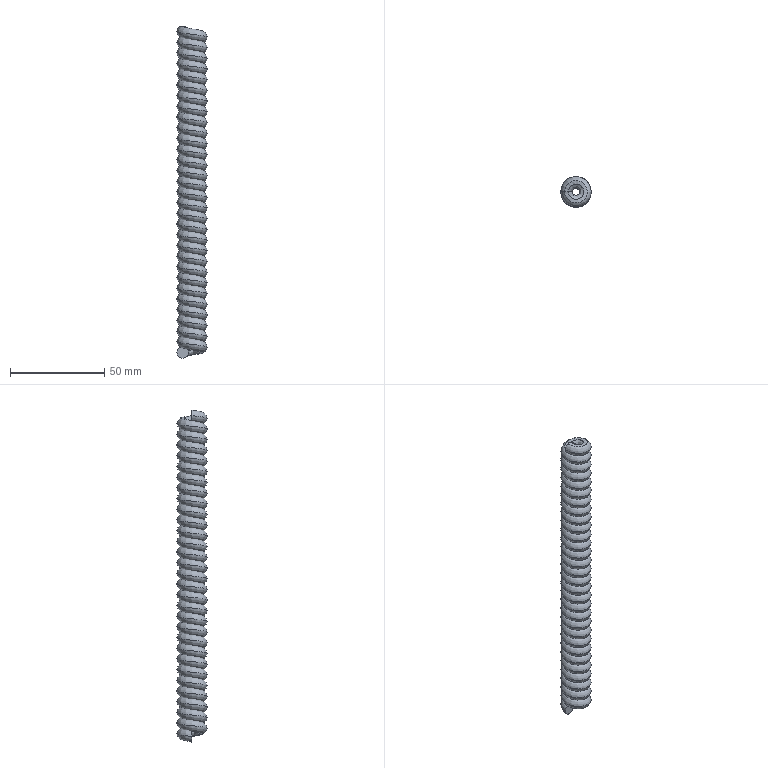Part | SolidWorks | features Helix 1, RefAxis 1, Sweep 1 | 1 solid | 8 faces | box 16 x 16 x 176 mm | volume 26240 mm3 | spline 6 | plane 2